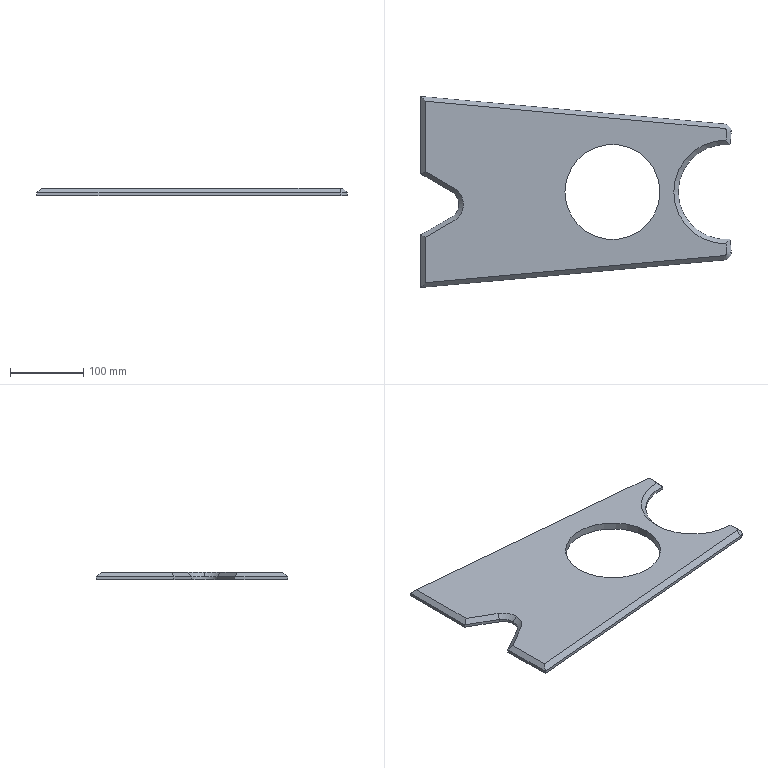Part | SolidWorks | features Chamfer 1, Extrusion 1 | 1 solid | 30 faces | box 424.836 x 261.6 x 10 mm | volume 684949 mm3 | plane 18 | cylinder 7 | cone 5 | commonest cylinder face diameters 130 x4 20 x2 40 x1
STEP:
#1=CARTESIAN_POINT('',(-210.073,-17.,4.));
#2=VERTEX_POINT('',#1);
#3=CARTESIAN_POINT('',(-220.073,0.3205,4.));
#4=VERTEX_POINT('',#3);
#5=CARTESIAN_POINT('',(-230.073,-17.,4.));
#6=DIRECTION('',(0.,0.,1.));
#7=DIRECTION('',(1.,0.,0.));
#8=AXIS2_PLACEMENT_3D('',#5,#6,#7);
#9=CIRCLE('',#8,20.);
#10=EDGE_CURVE('',#2,#4,#9,.T.);
#11=ORIENTED_EDGE('',*,*,#10,.F.);
#12=CARTESIAN_POINT('',(-204.073,-17.,10.));
#13=VERTEX_POINT('',#12);
#14=CARTESIAN_POINT('',(-204.073,-17.,10.));
#15=DIRECTION('',(0.7071,0.,0.7071));
#16=VECTOR('',#15,1000.);
#17=LINE('',#14,#16);
#18=EDGE_CURVE('',#2,#13,#17,.T.);
#19=ORIENTED_EDGE('',*,*,#18,.T.);
#20=CARTESIAN_POINT('',(-217.073,5.517,10.));
#21=VERTEX_POINT('',#20);
#22=CARTESIAN_POINT('',(-230.073,-17.,10.));
#23=DIRECTION('',(0.,0.,-1.));
#24=DIRECTION('',(1.,0.,0.));
#25=AXIS2_PLACEMENT_3D('',#22,#23,#24);
#26=CIRCLE('',#25,26.);
#27=EDGE_CURVE('',#21,#13,#26,.T.);
#28=ORIENTED_EDGE('',*,*,#27,.F.);
#29=CARTESIAN_POINT('',(-217.073,5.517,10.));
#30=DIRECTION('',(-0.3536,-0.6124,-0.7071));
#31=VECTOR('',#30,1000.);
#32=LINE('',#29,#31);
#33=EDGE_CURVE('',#21,#4,#32,.T.);
#34=ORIENTED_EDGE('',*,*,#33,.T.);
#35=EDGE_LOOP('',(#11,#19,#28,#34));
#36=FACE_OUTER_BOUND('',#35,.T.);
#37=CARTESIAN_POINT('',(-230.073,-17.,10.));
#38=DIRECTION('',(0.,0.,1.));
#39=DIRECTION('',(1.,0.,0.));
#40=AXIS2_PLACEMENT_3D('',#37,#38,#39);
#41=CONICAL_SURFACE('',#40,26.,0.7854);
#42=ADVANCED_FACE('',(#36),#41,.F.);
#43=CARTESIAN_POINT('',(-65.,0.,10.));
#44=VERTEX_POINT('',#43);
#45=CARTESIAN_POINT('',(65.,0.,10.));
#46=VERTEX_POINT('',#45);
#47=CARTESIAN_POINT('',(0.,0.,10.));
#48=DIRECTION('',(0.,0.,1.));
#49=DIRECTION('',(1.,0.,0.));
#50=AXIS2_PLACEMENT_3D('',#47,#48,#49);
#51=CIRCLE('',#50,65.);
#52=EDGE_CURVE('',#44,#46,#51,.T.);
#53=ORIENTED_EDGE('',*,*,#52,.T.);
#54=CARTESIAN_POINT('',(65.,0.,0.));
#55=VERTEX_POINT('',#54);
#56=CARTESIAN_POINT('',(65.,0.,10.));
#57=DIRECTION('',(0.,0.,-1.));
#58=VECTOR('',#57,1000.);
#59=LINE('',#56,#58);
#60=EDGE_CURVE('',#46,#55,#59,.T.);
#61=ORIENTED_EDGE('',*,*,#60,.T.);
#62=CARTESIAN_POINT('',(-65.,0.,0.));
#63=VERTEX_POINT('',#62);
#64=CARTESIAN_POINT('',(0.,0.,0.));
#65=DIRECTION('',(0.,0.,1.));
#66=DIRECTION('',(1.,0.,0.));
#67=AXIS2_PLACEMENT_3D('',#64,#65,#66);
#68=CIRCLE('',#67,65.);
#69=EDGE_CURVE('',#63,#55,#68,.T.);
#70=ORIENTED_EDGE('',*,*,#69,.F.);
#71=CARTESIAN_POINT('',(-65.,0.,10.));
#72=DIRECTION('',(0.,0.,-1.));
#73=VECTOR('',#72,1000.);
#74=LINE('',#71,#73);
#75=EDGE_CURVE('',#44,#63,#74,.T.);
#76=ORIENTED_EDGE('',*,*,#75,.F.);
#77=EDGE_LOOP('',(#53,#61,#70,#76));
#78=FACE_OUTER_BOUND('',#77,.T.);
#79=CARTESIAN_POINT('',(0.,0.,10.));
#80=DIRECTION('',(0.,0.,-1.));
#81=DIRECTION('',(-1.,0.,0.));
#82=AXIS2_PLACEMENT_3D('',#79,#80,#81);
#83=CYLINDRICAL_SURFACE('',#82,65.);
#84=ADVANCED_FACE('',(#78),#83,.F.);
#85=CARTESIAN_POINT('',(160.911,64.731,4.));
#86=VERTEX_POINT('',#85);
#87=CARTESIAN_POINT('',(90.,0.,4.));
#88=VERTEX_POINT('',#87);
#89=CARTESIAN_POINT('',(155.,0.,4.));
#90=DIRECTION('',(0.,0.,1.));
#91=DIRECTION('',(1.,0.,0.));
#92=AXIS2_PLACEMENT_3D('',#89,#90,#91);
#93=CIRCLE('',#92,65.);
#94=EDGE_CURVE('',#86,#88,#93,.T.);
#95=ORIENTED_EDGE('',*,*,#94,.T.);
#96=CARTESIAN_POINT('',(90.,0.,0.));
#97=VERTEX_POINT('',#96);
#98=CARTESIAN_POINT('',(90.,0.,10.));
#99=DIRECTION('',(0.,0.,-1.));
#100=VECTOR('',#99,1000.);
#101=LINE('',#98,#100);
#102=EDGE_CURVE('',#88,#97,#101,.T.);
#103=ORIENTED_EDGE('',*,*,#102,.T.);
#104=CARTESIAN_POINT('',(160.911,64.731,0.));
#105=VERTEX_POINT('',#104);
#106=CARTESIAN_POINT('',(155.,0.,0.));
#107=DIRECTION('',(0.,0.,-1.));
#108=DIRECTION('',(1.,0.,0.));
#109=AXIS2_PLACEMENT_3D('',#106,#107,#108);
#110=CIRCLE('',#109,65.);
#111=EDGE_CURVE('',#97,#105,#110,.T.);
#112=ORIENTED_EDGE('',*,*,#111,.T.);
#113=CARTESIAN_POINT('',(160.911,64.731,10.));
#114=DIRECTION('',(0.,0.,-1.));
#115=VECTOR('',#114,1000.);
#116=LINE('',#113,#115);
#117=EDGE_CURVE('',#86,#105,#116,.T.);
#118=ORIENTED_EDGE('',*,*,#117,.F.);
#119=EDGE_LOOP('',(#95,#103,#112,#118));
#120=FACE_OUTER_BOUND('',#119,.T.);
#121=CARTESIAN_POINT('',(155.,0.,10.));
#122=DIRECTION('',(0.,0.,-1.));
#123=DIRECTION('',(-1.,0.,0.));
#124=AXIS2_PLACEMENT_3D('',#121,#122,#123);
#125=CYLINDRICAL_SURFACE('',#124,65.);
#126=ADVANCED_FACE('',(#120),#125,.F.);
#127=CARTESIAN_POINT('',(152.898,-87.047,10.));
#128=VERTEX_POINT('',#127);
#129=CARTESIAN_POINT('',(156.52,-82.702,10.));
#130=VERTEX_POINT('',#129);
#131=CARTESIAN_POINT('',(152.536,-83.064,10.));
#132=DIRECTION('',(0.,0.,1.));
#133=DIRECTION('',(1.,0.,0.));
#134=AXIS2_PLACEMENT_3D('',#131,#132,#133);
#135=CIRCLE('',#134,4.);
#136=EDGE_CURVE('',#128,#130,#135,.T.);
#137=ORIENTED_EDGE('',*,*,#136,.T.);
#138=CARTESIAN_POINT('',(155.456,-70.999,10.));
#139=VERTEX_POINT('',#138);
#140=CARTESIAN_POINT('',(154.936,-65.274,10.));
#141=DIRECTION('',(-0.09049,0.9959,0.));
#142=VECTOR('',#141,1000.);
#143=LINE('',#140,#142);
#144=EDGE_CURVE('',#130,#139,#143,.T.);
#145=ORIENTED_EDGE('',*,*,#144,.T.);
#146=CARTESIAN_POINT('',(155.456,70.999,10.));
#147=VERTEX_POINT('',#146);
#148=CARTESIAN_POINT('',(155.,0.,10.));
#149=DIRECTION('',(0.,0.,-1.));
#150=DIRECTION('',(1.,0.,0.));
#151=AXIS2_PLACEMENT_3D('',#148,#149,#150);
#152=CIRCLE('',#151,71.);
#153=EDGE_CURVE('',#139,#147,#152,.T.);
#154=ORIENTED_EDGE('',*,*,#153,.T.);
#155=CARTESIAN_POINT('',(156.52,82.702,10.));
#156=VERTEX_POINT('',#155);
#157=CARTESIAN_POINT('',(156.52,82.702,10.));
#158=DIRECTION('',(0.09049,0.9959,0.));
#159=VECTOR('',#158,1000.);
#160=LINE('',#157,#159);
#161=EDGE_CURVE('',#147,#156,#160,.T.);
#162=ORIENTED_EDGE('',*,*,#161,.T.);
#163=CARTESIAN_POINT('',(152.898,87.047,10.));
#164=VERTEX_POINT('',#163);
#165=CARTESIAN_POINT('',(152.536,83.064,10.));
#166=DIRECTION('',(0.,0.,1.));
#167=DIRECTION('',(1.,0.,0.));
#168=AXIS2_PLACEMENT_3D('',#165,#166,#167);
#169=CIRCLE('',#168,4.);
#170=EDGE_CURVE('',#156,#164,#169,.T.);
#171=ORIENTED_EDGE('',*,*,#170,.T.);
#172=CARTESIAN_POINT('',(-256.3,124.23,10.));
#173=VERTEX_POINT('',#172);
#174=CARTESIAN_POINT('',(-262.843,124.825,10.));
#175=DIRECTION('',(-0.9959,0.09049,0.));
#176=VECTOR('',#175,1000.);
#177=LINE('',#174,#176);
#178=EDGE_CURVE('',#164,#173,#177,.T.);
#179=ORIENTED_EDGE('',*,*,#178,.T.);
#180=CARTESIAN_POINT('',(-256.3,28.164,10.));
#181=VERTEX_POINT('',#180);
#182=CARTESIAN_POINT('',(-256.3,24.7,10.));
#183=DIRECTION('',(0.,-1.,0.));
#184=VECTOR('',#183,1000.);
#185=LINE('',#182,#184);
#186=EDGE_CURVE('',#173,#181,#185,.T.);
#187=ORIENTED_EDGE('',*,*,#186,.T.);
#188=CARTESIAN_POINT('',(-217.073,5.517,10.));
#189=DIRECTION('',(0.866,-0.5,0.));
#190=VECTOR('',#189,1000.);
#191=LINE('',#188,#190);
#192=EDGE_CURVE('',#181,#21,#191,.T.);
#193=ORIENTED_EDGE('',*,*,#192,.T.);
#194=ORIENTED_EDGE('',*,*,#27,.T.);
#195=CARTESIAN_POINT('',(-217.073,-39.517,10.));
#196=VERTEX_POINT('',#195);
#197=CARTESIAN_POINT('',(-230.073,-17.,10.));
#198=DIRECTION('',(0.,0.,-1.));
#199=DIRECTION('',(1.,0.,0.));
#200=AXIS2_PLACEMENT_3D('',#197,#198,#199);
#201=CIRCLE('',#200,26.);
#202=EDGE_CURVE('',#13,#196,#201,.T.);
#203=ORIENTED_EDGE('',*,*,#202,.T.);
#204=CARTESIAN_POINT('',(-256.3,-62.164,10.));
#205=VERTEX_POINT('',#204);
#206=CARTESIAN_POINT('',(-259.3,-63.896,10.));
#207=DIRECTION('',(-0.866,-0.5,0.));
#208=VECTOR('',#207,1000.);
#209=LINE('',#206,#208);
#210=EDGE_CURVE('',#196,#205,#209,.T.);
#211=ORIENTED_EDGE('',*,*,#210,.T.);
#212=CARTESIAN_POINT('',(-256.3,-124.23,10.));
#213=VERTEX_POINT('',#212);
#214=CARTESIAN_POINT('',(-256.3,-130.8,10.));
#215=DIRECTION('',(0.,-1.,0.));
#216=VECTOR('',#215,1000.);
#217=LINE('',#214,#216);
#218=EDGE_CURVE('',#205,#213,#217,.T.);
#219=ORIENTED_EDGE('',*,*,#218,.T.);
#220=CARTESIAN_POINT('',(152.898,-87.047,10.));
#221=DIRECTION('',(0.9959,0.09049,0.));
#222=VECTOR('',#221,1000.);
#223=LINE('',#220,#222);
#224=EDGE_CURVE('',#213,#128,#223,.T.);
#225=ORIENTED_EDGE('',*,*,#224,.T.);
#226=EDGE_LOOP('',(#137,#145,#154,#162,#171,#179,#187,#193,#194,#203,#211,#219,#225));
#227=FACE_OUTER_BOUND('',#226,.T.);
#228=ORIENTED_EDGE('',*,*,#52,.F.);
#229=CARTESIAN_POINT('',(0.,0.,10.));
#230=DIRECTION('',(0.,0.,1.));
#231=DIRECTION('',(1.,0.,0.));
#232=AXIS2_PLACEMENT_3D('',#229,#230,#231);
#233=CIRCLE('',#232,65.);
#234=EDGE_CURVE('',#46,#44,#233,.T.);
#235=ORIENTED_EDGE('',*,*,#234,.F.);
#236=EDGE_LOOP('',(#228,#235));
#237=FACE_BOUND('',#236,.T.);
#238=CARTESIAN_POINT('',(152.536,-83.064,10.));
#239=DIRECTION('',(0.,0.,1.));
#240=DIRECTION('',(1.,0.,0.));
#241=AXIS2_PLACEMENT_3D('',#238,#239,#240);
#242=PLANE('',#241);
#243=ADVANCED_FACE('',(#227,#237),#242,.T.);
#244=CARTESIAN_POINT('',(-262.3,-58.7,0.));
#245=VERTEX_POINT('',#244);
#246=CARTESIAN_POINT('',(-262.3,-130.8,0.));
#247=VERTEX_POINT('',#246);
#248=CARTESIAN_POINT('',(-262.3,-58.7,0.));
#249=DIRECTION('',(0.,-1.,0.));
#250=VECTOR('',#249,1000.);
#251=LINE('',#248,#250);
#252=EDGE_CURVE('',#245,#247,#251,.T.);
#253=ORIENTED_EDGE('',*,*,#252,.F.);
#254=CARTESIAN_POINT('',(-220.073,-34.321,0.));
#255=VERTEX_POINT('',#254);
#256=CARTESIAN_POINT('',(-262.3,-58.7,0.));
#257=DIRECTION('',(-0.866,-0.5,0.));
#258=VECTOR('',#257,1000.);
#259=LINE('',#256,#258);
#260=EDGE_CURVE('',#255,#245,#259,.T.);
#261=ORIENTED_EDGE('',*,*,#260,.F.);
#262=CARTESIAN_POINT('',(-220.073,0.3205,0.));
#263=VERTEX_POINT('',#262);
#264=CARTESIAN_POINT('',(-230.073,-17.,0.));
#265=DIRECTION('',(0.,0.,-1.));
#266=DIRECTION('',(-1.,0.,0.));
#267=AXIS2_PLACEMENT_3D('',#264,#265,#266);
#268=CIRCLE('',#267,20.);
#269=EDGE_CURVE('',#263,#255,#268,.T.);
#270=ORIENTED_EDGE('',*,*,#269,.F.);
#271=CARTESIAN_POINT('',(-262.3,24.7,0.));
#272=VERTEX_POINT('',#271);
#273=CARTESIAN_POINT('',(-262.3,24.7,0.));
#274=DIRECTION('',(0.866,-0.5,0.));
#275=VECTOR('',#274,1000.);
#276=LINE('',#273,#275);
#277=EDGE_CURVE('',#272,#263,#276,.T.);
#278=ORIENTED_EDGE('',*,*,#277,.F.);
#279=CARTESIAN_POINT('',(-262.3,130.8,0.));
#280=VERTEX_POINT('',#279);
#281=CARTESIAN_POINT('',(-262.3,130.8,0.));
#282=DIRECTION('',(0.,-1.,0.));
#283=VECTOR('',#282,1000.);
#284=LINE('',#281,#283);
#285=EDGE_CURVE('',#280,#272,#284,.T.);
#286=ORIENTED_EDGE('',*,*,#285,.F.);
#287=CARTESIAN_POINT('',(153.441,93.023,0.));
#288=VERTEX_POINT('',#287);
#289=CARTESIAN_POINT('',(-262.3,130.8,0.));
#290=DIRECTION('',(-0.9959,0.09049,0.));
#291=VECTOR('',#290,1000.);
#292=LINE('',#289,#291);
#293=EDGE_CURVE('',#288,#280,#292,.T.);
#294=ORIENTED_EDGE('',*,*,#293,.F.);
#295=CARTESIAN_POINT('',(162.495,82.159,0.));
#296=VERTEX_POINT('',#295);
#297=CARTESIAN_POINT('',(152.536,83.064,0.));
#298=DIRECTION('',(0.,0.,1.));
#299=DIRECTION('',(-1.,0.,0.));
#300=AXIS2_PLACEMENT_3D('',#297,#298,#299);
#301=CIRCLE('',#300,10.);
#302=EDGE_CURVE('',#296,#288,#301,.T.);
#303=ORIENTED_EDGE('',*,*,#302,.F.);
#304=CARTESIAN_POINT('',(162.495,82.159,0.));
#305=DIRECTION('',(0.09049,0.9959,0.));
#306=VECTOR('',#305,1000.);
#307=LINE('',#304,#306);
#308=EDGE_CURVE('',#105,#296,#307,.T.);
#309=ORIENTED_EDGE('',*,*,#308,.F.);
#310=ORIENTED_EDGE('',*,*,#111,.F.);
#311=CARTESIAN_POINT('',(160.911,-64.731,0.));
#312=VERTEX_POINT('',#311);
#313=CARTESIAN_POINT('',(155.,0.,0.));
#314=DIRECTION('',(0.,0.,-1.));
#315=DIRECTION('',(1.,0.,0.));
#316=AXIS2_PLACEMENT_3D('',#313,#314,#315);
#317=CIRCLE('',#316,65.);
#318=EDGE_CURVE('',#312,#97,#317,.T.);
#319=ORIENTED_EDGE('',*,*,#318,.F.);
#320=CARTESIAN_POINT('',(162.495,-82.159,0.));
#321=VERTEX_POINT('',#320);
#322=CARTESIAN_POINT('',(162.495,-82.159,0.));
#323=DIRECTION('',(-0.09049,0.9959,0.));
#324=VECTOR('',#323,1000.);
#325=LINE('',#322,#324);
#326=EDGE_CURVE('',#321,#312,#325,.T.);
#327=ORIENTED_EDGE('',*,*,#326,.F.);
#328=CARTESIAN_POINT('',(153.441,-93.023,0.));
#329=VERTEX_POINT('',#328);
#330=CARTESIAN_POINT('',(152.536,-83.064,0.));
#331=DIRECTION('',(0.,0.,1.));
#332=DIRECTION('',(1.,0.,0.));
#333=AXIS2_PLACEMENT_3D('',#330,#331,#332);
#334=CIRCLE('',#333,10.);
#335=EDGE_CURVE('',#329,#321,#334,.T.);
#336=ORIENTED_EDGE('',*,*,#335,.F.);
#337=CARTESIAN_POINT('',(-262.3,-130.8,0.));
#338=DIRECTION('',(0.9959,0.09049,0.));
#339=VECTOR('',#338,1000.);
#340=LINE('',#337,#339);
#341=EDGE_CURVE('',#247,#329,#340,.T.);
#342=ORIENTED_EDGE('',*,*,#341,.F.);
#343=EDGE_LOOP('',(#253,#261,#270,#278,#286,#294,#303,#309,#310,#319,#327,#336,#342));
#344=FACE_OUTER_BOUND('',#343,.T.);
#345=ORIENTED_EDGE('',*,*,#69,.T.);
#346=CARTESIAN_POINT('',(0.,0.,0.));
#347=DIRECTION('',(0.,0.,1.));
#348=DIRECTION('',(1.,0.,0.));
#349=AXIS2_PLACEMENT_3D('',#346,#347,#348);
#350=CIRCLE('',#349,65.);
#351=EDGE_CURVE('',#55,#63,#350,.T.);
#352=ORIENTED_EDGE('',*,*,#351,.T.);
#353=EDGE_LOOP('',(#345,#352));
#354=FACE_BOUND('',#353,.T.);
#355=CARTESIAN_POINT('',(152.536,-83.064,0.));
#356=DIRECTION('',(0.,0.,1.));
#357=DIRECTION('',(1.,0.,0.));
#358=AXIS2_PLACEMENT_3D('',#355,#356,#357);
#359=PLANE('',#358);
#360=ADVANCED_FACE('',(#344,#354),#359,.F.);
#361=CARTESIAN_POINT('',(-262.3,-130.8,4.));
#362=VERTEX_POINT('',#361);
#363=CARTESIAN_POINT('',(-262.3,-130.8,10.));
#364=DIRECTION('',(0.,0.,-1.));
#365=VECTOR('',#364,1000.);
#366=LINE('',#363,#365);
#367=EDGE_CURVE('',#362,#247,#366,.T.);
#368=ORIENTED_EDGE('',*,*,#367,.F.);
#369=CARTESIAN_POINT('',(-262.3,-58.7,4.));
#370=VERTEX_POINT('',#369);
#371=CARTESIAN_POINT('',(-262.3,-58.7,4.));
#372=DIRECTION('',(0.,1.,0.));
#373=VECTOR('',#372,1000.);
#374=LINE('',#371,#373);
#375=EDGE_CURVE('',#362,#370,#374,.T.);
#376=ORIENTED_EDGE('',*,*,#375,.T.);
#377=CARTESIAN_POINT('',(-262.3,-58.7,10.));
#378=DIRECTION('',(0.,0.,-1.));
#379=VECTOR('',#378,1000.);
#380=LINE('',#377,#379);
#381=EDGE_CURVE('',#370,#245,#380,.T.);
#382=ORIENTED_EDGE('',*,*,#381,.T.);
#383=ORIENTED_EDGE('',*,*,#252,.T.);
#384=EDGE_LOOP('',(#368,#376,#382,#383));
#385=FACE_OUTER_BOUND('',#384,.T.);
#386=CARTESIAN_POINT('',(-262.3,-58.7,10.));
#387=DIRECTION('',(1.,0.,0.));
#388=DIRECTION('',(0.,1.,0.));
#389=AXIS2_PLACEMENT_3D('',#386,#387,#388);
#390=PLANE('',#389);
#391=ADVANCED_FACE('',(#385),#390,.F.);
#392=CARTESIAN_POINT('',(153.441,-93.023,4.));
#393=VERTEX_POINT('',#392);
#394=CARTESIAN_POINT('',(153.441,-93.023,10.));
#395=DIRECTION('',(0.,0.,-1.));
#396=VECTOR('',#395,1000.);
#397=LINE('',#394,#396);
#398=EDGE_CURVE('',#393,#329,#397,.T.);
#399=ORIENTED_EDGE('',*,*,#398,.F.);
#400=CARTESIAN_POINT('',(-262.3,-130.8,4.));
#401=DIRECTION('',(-0.9959,-0.09049,0.));
#402=VECTOR('',#401,1000.);
#403=LINE('',#400,#402);
#404=EDGE_CURVE('',#393,#362,#403,.T.);
#405=ORIENTED_EDGE('',*,*,#404,.T.);
#406=ORIENTED_EDGE('',*,*,#367,.T.);
#407=ORIENTED_EDGE('',*,*,#341,.T.);
#408=EDGE_LOOP('',(#399,#405,#406,#407));
#409=FACE_OUTER_BOUND('',#408,.T.);
#410=CARTESIAN_POINT('',(-262.3,-130.8,10.));
#411=DIRECTION('',(-0.09049,0.9959,0.));
#412=DIRECTION('',(-0.9959,-0.09049,0.));
#413=AXIS2_PLACEMENT_3D('',#410,#411,#412);
#414=PLANE('',#413);
#415=ADVANCED_FACE('',(#409),#414,.F.);
#416=CARTESIAN_POINT('',(162.495,-82.159,4.));
#417=VERTEX_POINT('',#416);
#418=CARTESIAN_POINT('',(162.495,-82.159,10.));
#419=DIRECTION('',(0.,0.,-1.));
#420=VECTOR('',#419,1000.);
#421=LINE('',#418,#420);
#422=EDGE_CURVE('',#417,#321,#421,.T.);
#423=ORIENTED_EDGE('',*,*,#422,.F.);
#424=CARTESIAN_POINT('',(152.536,-83.064,4.));
#425=DIRECTION('',(0.,0.,-1.));
#426=DIRECTION('',(1.,0.,0.));
#427=AXIS2_PLACEMENT_3D('',#424,#425,#426);
#428=CIRCLE('',#427,10.);
#429=EDGE_CURVE('',#417,#393,#428,.T.);
#430=ORIENTED_EDGE('',*,*,#429,.T.);
#431=ORIENTED_EDGE('',*,*,#398,.T.);
#432=ORIENTED_EDGE('',*,*,#335,.T.);
#433=EDGE_LOOP('',(#423,#430,#431,#432));
#434=FACE_OUTER_BOUND('',#433,.T.);
#435=CARTESIAN_POINT('',(152.536,-83.064,10.));
#436=DIRECTION('',(0.,0.,-1.));
#437=DIRECTION('',(-1.,0.,0.));
#438=AXIS2_PLACEMENT_3D('',#435,#436,#437);
#439=CYLINDRICAL_SURFACE('',#438,10.);
#440=ADVANCED_FACE('',(#434),#439,.T.);
#441=CARTESIAN_POINT('',(160.911,-64.731,4.));
#442=VERTEX_POINT('',#441);
#443=CARTESIAN_POINT('',(160.911,-64.731,10.));
#444=DIRECTION('',(0.,0.,-1.));
#445=VECTOR('',#444,1000.);
#446=LINE('',#443,#445);
#447=EDGE_CURVE('',#442,#312,#446,.T.);
#448=ORIENTED_EDGE('',*,*,#447,.F.);
#449=CARTESIAN_POINT('',(162.495,-82.159,4.));
#450=DIRECTION('',(0.09049,-0.9959,0.));
#451=VECTOR('',#450,1000.);
#452=LINE('',#449,#451);
#453=EDGE_CURVE('',#442,#417,#452,.T.);
#454=ORIENTED_EDGE('',*,*,#453,.T.);
#455=ORIENTED_EDGE('',*,*,#422,.T.);
#456=ORIENTED_EDGE('',*,*,#326,.T.);
#457=EDGE_LOOP('',(#448,#454,#455,#456));
#458=FACE_OUTER_BOUND('',#457,.T.);
#459=CARTESIAN_POINT('',(162.495,-82.159,10.));
#460=DIRECTION('',(-0.9959,-0.09049,0.));
#461=DIRECTION('',(0.09049,-0.9959,0.));
#462=AXIS2_PLACEMENT_3D('',#459,#460,#461);
#463=PLANE('',#462);
#464=ADVANCED_FACE('',(#458),#463,.F.);
#465=ORIENTED_EDGE('',*,*,#102,.F.);
#466=CARTESIAN_POINT('',(155.,0.,4.));
#467=DIRECTION('',(0.,0.,1.));
#468=DIRECTION('',(1.,0.,0.));
#469=AXIS2_PLACEMENT_3D('',#466,#467,#468);
#470=CIRCLE('',#469,65.);
#471=EDGE_CURVE('',#88,#442,#470,.T.);
#472=ORIENTED_EDGE('',*,*,#471,.T.);
#473=ORIENTED_EDGE('',*,*,#447,.T.);
#474=ORIENTED_EDGE('',*,*,#318,.T.);
#475=EDGE_LOOP('',(#465,#472,#473,#474));
#476=FACE_OUTER_BOUND('',#475,.T.);
#477=CARTESIAN_POINT('',(155.,0.,10.));
#478=DIRECTION('',(0.,0.,-1.));
#479=DIRECTION('',(-1.,0.,0.));
#480=AXIS2_PLACEMENT_3D('',#477,#478,#479);
#481=CYLINDRICAL_SURFACE('',#480,65.);
#482=ADVANCED_FACE('',(#476),#481,.F.);
#483=CARTESIAN_POINT('',(162.495,82.159,4.));
#484=VERTEX_POINT('',#483);
#485=CARTESIAN_POINT('',(162.495,82.159,10.));
#486=DIRECTION('',(0.,0.,-1.));
#487=VECTOR('',#486,1000.);
#488=LINE('',#485,#487);
#489=EDGE_CURVE('',#484,#296,#488,.T.);
#490=ORIENTED_EDGE('',*,*,#489,.F.);
#491=CARTESIAN_POINT('',(160.911,64.731,4.));
#492=DIRECTION('',(-0.09049,-0.9959,0.));
#493=VECTOR('',#492,1000.);
#494=LINE('',#491,#493);
#495=EDGE_CURVE('',#484,#86,#494,.T.);
#496=ORIENTED_EDGE('',*,*,#495,.T.);
#497=ORIENTED_EDGE('',*,*,#117,.T.);
#498=ORIENTED_EDGE('',*,*,#308,.T.);
#499=EDGE_LOOP('',(#490,#496,#497,#498));
#500=FACE_OUTER_BOUND('',#499,.T.);
#501=CARTESIAN_POINT('',(162.495,82.159,10.));
#502=DIRECTION('',(-0.9959,0.09049,0.));
#503=DIRECTION('',(-0.09049,-0.9959,0.));
#504=AXIS2_PLACEMENT_3D('',#501,#502,#503);
#505=PLANE('',#504);
#506=ADVANCED_FACE('',(#500),#505,.F.);
#507=CARTESIAN_POINT('',(153.441,93.023,4.));
#508=VERTEX_POINT('',#507);
#509=CARTESIAN_POINT('',(153.441,93.023,10.));
#510=DIRECTION('',(0.,0.,-1.));
#511=VECTOR('',#510,1000.);
#512=LINE('',#509,#511);
#513=EDGE_CURVE('',#508,#288,#512,.T.);
#514=ORIENTED_EDGE('',*,*,#513,.F.);
#515=CARTESIAN_POINT('',(152.536,83.064,4.));
#516=DIRECTION('',(0.,0.,-1.));
#517=DIRECTION('',(1.,0.,0.));
#518=AXIS2_PLACEMENT_3D('',#515,#516,#517);
#519=CIRCLE('',#518,10.);
#520=EDGE_CURVE('',#508,#484,#519,.T.);
#521=ORIENTED_EDGE('',*,*,#520,.T.);
#522=ORIENTED_EDGE('',*,*,#489,.T.);
#523=ORIENTED_EDGE('',*,*,#302,.T.);
#524=EDGE_LOOP('',(#514,#521,#522,#523));
#525=FACE_OUTER_BOUND('',#524,.T.);
#526=CARTESIAN_POINT('',(152.536,83.064,10.));
#527=DIRECTION('',(0.,0.,-1.));
#528=DIRECTION('',(-1.,0.,0.));
#529=AXIS2_PLACEMENT_3D('',#526,#527,#528);
#530=CYLINDRICAL_SURFACE('',#529,10.);
#531=ADVANCED_FACE('',(#525),#530,.T.);
#532=CARTESIAN_POINT('',(-262.3,130.8,4.));
#533=VERTEX_POINT('',#532);
#534=CARTESIAN_POINT('',(-262.3,130.8,10.));
#535=DIRECTION('',(0.,0.,-1.));
#536=VECTOR('',#535,1000.);
#537=LINE('',#534,#536);
#538=EDGE_CURVE('',#533,#280,#537,.T.);
#539=ORIENTED_EDGE('',*,*,#538,.F.);
#540=CARTESIAN_POINT('',(153.441,93.023,4.));
#541=DIRECTION('',(0.9959,-0.09049,0.));
#542=VECTOR('',#541,1000.);
#543=LINE('',#540,#542);
#544=EDGE_CURVE('',#533,#508,#543,.T.);
#545=ORIENTED_EDGE('',*,*,#544,.T.);
#546=ORIENTED_EDGE('',*,*,#513,.T.);
#547=ORIENTED_EDGE('',*,*,#293,.T.);
#548=EDGE_LOOP('',(#539,#545,#546,#547));
#549=FACE_OUTER_BOUND('',#548,.T.);
#550=CARTESIAN_POINT('',(-262.3,130.8,10.));
#551=DIRECTION('',(-0.09049,-0.9959,0.));
#552=DIRECTION('',(0.9959,-0.09049,0.));
#553=AXIS2_PLACEMENT_3D('',#550,#551,#552);
#554=PLANE('',#553);
#555=ADVANCED_FACE('',(#549),#554,.F.);
#556=CARTESIAN_POINT('',(-262.3,24.7,4.));
#557=VERTEX_POINT('',#556);
#558=CARTESIAN_POINT('',(-262.3,24.7,10.));
#559=DIRECTION('',(0.,0.,-1.));
#560=VECTOR('',#559,1000.);
#561=LINE('',#558,#560);
#562=EDGE_CURVE('',#557,#272,#561,.T.);
#563=ORIENTED_EDGE('',*,*,#562,.F.);
#564=CARTESIAN_POINT('',(-262.3,130.8,4.));
#565=DIRECTION('',(0.,1.,0.));
#566=VECTOR('',#565,1000.);
#567=LINE('',#564,#566);
#568=EDGE_CURVE('',#557,#533,#567,.T.);
#569=ORIENTED_EDGE('',*,*,#568,.T.);
#570=ORIENTED_EDGE('',*,*,#538,.T.);
#571=ORIENTED_EDGE('',*,*,#285,.T.);
#572=EDGE_LOOP('',(#563,#569,#570,#571));
#573=FACE_OUTER_BOUND('',#572,.T.);
#574=CARTESIAN_POINT('',(-262.3,130.8,10.));
#575=DIRECTION('',(1.,0.,0.));
#576=DIRECTION('',(0.,1.,0.));
#577=AXIS2_PLACEMENT_3D('',#574,#575,#576);
#578=PLANE('',#577);
#579=ADVANCED_FACE('',(#573),#578,.F.);
#580=CARTESIAN_POINT('',(-220.073,0.3205,10.));
#581=DIRECTION('',(0.,0.,-1.));
#582=VECTOR('',#581,1000.);
#583=LINE('',#580,#582);
#584=EDGE_CURVE('',#4,#263,#583,.T.);
#585=ORIENTED_EDGE('',*,*,#584,.F.);
#586=CARTESIAN_POINT('',(-262.3,24.7,4.));
#587=DIRECTION('',(-0.866,0.5,0.));
#588=VECTOR('',#587,1000.);
#589=LINE('',#586,#588);
#590=EDGE_CURVE('',#4,#557,#589,.T.);
#591=ORIENTED_EDGE('',*,*,#590,.T.);
#592=ORIENTED_EDGE('',*,*,#562,.T.);
#593=ORIENTED_EDGE('',*,*,#277,.T.);
#594=EDGE_LOOP('',(#585,#591,#592,#593));
#595=FACE_OUTER_BOUND('',#594,.T.);
#596=CARTESIAN_POINT('',(-262.3,24.7,10.));
#597=DIRECTION('',(0.5,0.866,0.));
#598=DIRECTION('',(-0.866,0.5,0.));
#599=AXIS2_PLACEMENT_3D('',#596,#597,#598);
#600=PLANE('',#599);
#601=ADVANCED_FACE('',(#595),#600,.F.);
#602=CARTESIAN_POINT('',(-220.073,-34.321,4.));
#603=VERTEX_POINT('',#602);
#604=CARTESIAN_POINT('',(-220.073,-34.321,10.));
#605=DIRECTION('',(0.,0.,-1.));
#606=VECTOR('',#605,1000.);
#607=LINE('',#604,#606);
#608=EDGE_CURVE('',#603,#255,#607,.T.);
#609=ORIENTED_EDGE('',*,*,#608,.F.);
#610=CARTESIAN_POINT('',(-230.073,-17.,4.));
#611=DIRECTION('',(0.,0.,1.));
#612=DIRECTION('',(1.,0.,0.));
#613=AXIS2_PLACEMENT_3D('',#610,#611,#612);
#614=CIRCLE('',#613,20.);
#615=EDGE_CURVE('',#603,#2,#614,.T.);
#616=ORIENTED_EDGE('',*,*,#615,.T.);
#617=ORIENTED_EDGE('',*,*,#10,.T.);
#618=ORIENTED_EDGE('',*,*,#584,.T.);
#619=ORIENTED_EDGE('',*,*,#269,.T.);
#620=EDGE_LOOP('',(#609,#616,#617,#618,#619));
#621=FACE_OUTER_BOUND('',#620,.T.);
#622=CARTESIAN_POINT('',(-230.073,-17.,10.));
#623=DIRECTION('',(0.,0.,-1.));
#624=DIRECTION('',(-1.,0.,0.));
#625=AXIS2_PLACEMENT_3D('',#622,#623,#624);
#626=CYLINDRICAL_SURFACE('',#625,20.);
#627=ADVANCED_FACE('',(#621),#626,.F.);
#628=ORIENTED_EDGE('',*,*,#381,.F.);
#629=CARTESIAN_POINT('',(-220.073,-34.321,4.));
#630=DIRECTION('',(0.866,0.5,0.));
#631=VECTOR('',#630,1000.);
#632=LINE('',#629,#631);
#633=EDGE_CURVE('',#370,#603,#632,.T.);
#634=ORIENTED_EDGE('',*,*,#633,.T.);
#635=ORIENTED_EDGE('',*,*,#608,.T.);
#636=ORIENTED_EDGE('',*,*,#260,.T.);
#637=EDGE_LOOP('',(#628,#634,#635,#636));
#638=FACE_OUTER_BOUND('',#637,.T.);
#639=CARTESIAN_POINT('',(-262.3,-58.7,10.));
#640=DIRECTION('',(0.5,-0.866,0.));
#641=DIRECTION('',(0.866,0.5,0.));
#642=AXIS2_PLACEMENT_3D('',#639,#640,#641);
#643=PLANE('',#642);
#644=ADVANCED_FACE('',(#638),#643,.F.);
#645=ORIENTED_EDGE('',*,*,#60,.F.);
#646=ORIENTED_EDGE('',*,*,#234,.T.);
#647=ORIENTED_EDGE('',*,*,#75,.T.);
#648=ORIENTED_EDGE('',*,*,#351,.F.);
#649=EDGE_LOOP('',(#645,#646,#647,#648));
#650=FACE_OUTER_BOUND('',#649,.T.);
#651=CARTESIAN_POINT('',(0.,0.,10.));
#652=DIRECTION('',(0.,0.,-1.));
#653=DIRECTION('',(-1.,0.,0.));
#654=AXIS2_PLACEMENT_3D('',#651,#652,#653);
#655=CYLINDRICAL_SURFACE('',#654,65.);
#656=ADVANCED_FACE('',(#650),#655,.F.);
#657=CARTESIAN_POINT('',(-283.822,12.274,-17.522));
#658=DIRECTION('',(0.6547,0.378,0.6547));
#659=VECTOR('',#658,1000.);
#660=LINE('',#657,#659);
#661=EDGE_CURVE('',#557,#181,#660,.T.);
#662=ORIENTED_EDGE('',*,*,#661,.F.);
#663=ORIENTED_EDGE('',*,*,#590,.F.);
#664=ORIENTED_EDGE('',*,*,#33,.F.);
#665=ORIENTED_EDGE('',*,*,#192,.F.);
#666=EDGE_LOOP('',(#662,#663,#664,#665));
#667=FACE_OUTER_BOUND('',#666,.T.);
#668=CARTESIAN_POINT('',(98.49,-176.674,10.));
#669=DIRECTION('',(-0.3536,-0.6124,0.7071));
#670=DIRECTION('',(0.,-0.7559,-0.6547));
#671=AXIS2_PLACEMENT_3D('',#668,#669,#670);
#672=PLANE('',#671);
#673=ADVANCED_FACE('',(#667),#672,.T.);
#674=ORIENTED_EDGE('',*,*,#18,.F.);
#675=ORIENTED_EDGE('',*,*,#615,.F.);
#676=CARTESIAN_POINT('',(-217.073,-39.517,10.));
#677=DIRECTION('',(-0.3536,0.6124,-0.7071));
#678=VECTOR('',#677,1000.);
#679=LINE('',#676,#678);
#680=EDGE_CURVE('',#196,#603,#679,.T.);
#681=ORIENTED_EDGE('',*,*,#680,.F.);
#682=ORIENTED_EDGE('',*,*,#202,.F.);
#683=EDGE_LOOP('',(#674,#675,#681,#682));
#684=FACE_OUTER_BOUND('',#683,.T.);
#685=CARTESIAN_POINT('',(-230.073,-17.,10.));
#686=DIRECTION('',(0.,0.,1.));
#687=DIRECTION('',(1.,0.,0.));
#688=AXIS2_PLACEMENT_3D('',#685,#686,#687);
#689=CONICAL_SURFACE('',#688,26.,0.7854);
#690=ADVANCED_FACE('',(#684),#689,.F.);
#691=ORIENTED_EDGE('',*,*,#661,.T.);
#692=ORIENTED_EDGE('',*,*,#186,.F.);
#693=CARTESIAN_POINT('',(-110.512,-35.406,155.788));
#694=DIRECTION('',(0.5591,-0.6122,0.5591));
#695=VECTOR('',#694,1000.);
#696=LINE('',#693,#695);
#697=EDGE_CURVE('',#533,#173,#696,.T.);
#698=ORIENTED_EDGE('',*,*,#697,.F.);
#699=ORIENTED_EDGE('',*,*,#568,.F.);
#700=EDGE_LOOP('',(#691,#692,#698,#699));
#701=FACE_OUTER_BOUND('',#700,.T.);
#702=CARTESIAN_POINT('',(-256.3,-83.064,10.));
#703=DIRECTION('',(-0.7071,0.,0.7071));
#704=DIRECTION('',(0.7071,0.,0.7071));
#705=AXIS2_PLACEMENT_3D('',#702,#703,#704);
#706=PLANE('',#705);
#707=ADVANCED_FACE('',(#701),#706,.T.);
#708=ORIENTED_EDGE('',*,*,#680,.T.);
#709=ORIENTED_EDGE('',*,*,#633,.F.);
#710=CARTESIAN_POINT('',(-171.278,-111.252,95.022));
#711=DIRECTION('',(-0.6547,0.378,-0.6547));
#712=VECTOR('',#711,1000.);
#713=LINE('',#710,#712);
#714=EDGE_CURVE('',#205,#370,#713,.T.);
#715=ORIENTED_EDGE('',*,*,#714,.F.);
#716=ORIENTED_EDGE('',*,*,#210,.F.);
#717=EDGE_LOOP('',(#708,#709,#715,#716));
#718=FACE_OUTER_BOUND('',#717,.T.);
#719=CARTESIAN_POINT('',(41.277,109.642,10.));
#720=DIRECTION('',(-0.3536,0.6124,0.7071));
#721=DIRECTION('',(0.,-0.7559,0.6547));
#722=AXIS2_PLACEMENT_3D('',#719,#720,#721);
#723=PLANE('',#722);
#724=ADVANCED_FACE('',(#718),#723,.T.);
#725=ORIENTED_EDGE('',*,*,#697,.T.);
#726=ORIENTED_EDGE('',*,*,#178,.F.);
#727=CARTESIAN_POINT('',(153.441,93.023,4.));
#728=DIRECTION('',(-0.06399,-0.7042,0.7071));
#729=VECTOR('',#728,1000.);
#730=LINE('',#727,#729);
#731=EDGE_CURVE('',#508,#164,#730,.T.);
#732=ORIENTED_EDGE('',*,*,#731,.F.);
#733=ORIENTED_EDGE('',*,*,#544,.F.);
#734=EDGE_LOOP('',(#725,#726,#732,#733));
#735=FACE_OUTER_BOUND('',#734,.T.);
#736=CARTESIAN_POINT('',(167.87,85.687,10.));
#737=DIRECTION('',(0.06399,0.7042,0.7071));
#738=DIRECTION('',(0.,-0.7086,0.7057));
#739=AXIS2_PLACEMENT_3D('',#736,#737,#738);
#740=PLANE('',#739);
#741=ADVANCED_FACE('',(#735),#740,.T.);
#742=ORIENTED_EDGE('',*,*,#714,.T.);
#743=ORIENTED_EDGE('',*,*,#375,.F.);
#744=CARTESIAN_POINT('',(-242.209,-108.801,24.091));
#745=DIRECTION('',(-0.5591,-0.6122,-0.5591));
#746=VECTOR('',#745,1000.);
#747=LINE('',#744,#746);
#748=EDGE_CURVE('',#213,#362,#747,.T.);
#749=ORIENTED_EDGE('',*,*,#748,.F.);
#750=ORIENTED_EDGE('',*,*,#218,.F.);
#751=EDGE_LOOP('',(#742,#743,#749,#750));
#752=FACE_OUTER_BOUND('',#751,.T.);
#753=CARTESIAN_POINT('',(-256.3,-83.064,10.));
#754=DIRECTION('',(-0.7071,0.,0.7071));
#755=DIRECTION('',(0.7071,0.,0.7071));
#756=AXIS2_PLACEMENT_3D('',#753,#754,#755);
#757=PLANE('',#756);
#758=ADVANCED_FACE('',(#752),#757,.T.);
#759=ORIENTED_EDGE('',*,*,#731,.T.);
#760=ORIENTED_EDGE('',*,*,#170,.F.);
#761=CARTESIAN_POINT('',(162.495,82.159,4.));
#762=DIRECTION('',(-0.7042,0.06399,0.7071));
#763=VECTOR('',#762,1000.);
#764=LINE('',#761,#763);
#765=EDGE_CURVE('',#484,#156,#764,.T.);
#766=ORIENTED_EDGE('',*,*,#765,.F.);
#767=ORIENTED_EDGE('',*,*,#520,.F.);
#768=EDGE_LOOP('',(#759,#760,#766,#767));
#769=FACE_OUTER_BOUND('',#768,.T.);
#770=CARTESIAN_POINT('',(152.536,83.064,10.));
#771=DIRECTION('',(0.,0.,-1.));
#772=DIRECTION('',(-1.,0.,0.));
#773=AXIS2_PLACEMENT_3D('',#770,#771,#772);
#774=CONICAL_SURFACE('',#773,4.,0.7854);
#775=ADVANCED_FACE('',(#769),#774,.T.);
#776=ORIENTED_EDGE('',*,*,#748,.T.);
#777=ORIENTED_EDGE('',*,*,#404,.F.);
#778=CARTESIAN_POINT('',(152.898,-87.047,10.));
#779=DIRECTION('',(0.06399,-0.7042,-0.7071));
#780=VECTOR('',#779,1000.);
#781=LINE('',#778,#780);
#782=EDGE_CURVE('',#128,#393,#781,.T.);
#783=ORIENTED_EDGE('',*,*,#782,.F.);
#784=ORIENTED_EDGE('',*,*,#224,.F.);
#785=EDGE_LOOP('',(#776,#777,#783,#784));
#786=FACE_OUTER_BOUND('',#785,.T.);
#787=CARTESIAN_POINT('',(152.898,-87.047,10.));
#788=DIRECTION('',(0.06399,-0.7042,0.7071));
#789=DIRECTION('',(0.,-0.7086,-0.7057));
#790=AXIS2_PLACEMENT_3D('',#787,#788,#789);
#791=PLANE('',#790);
#792=ADVANCED_FACE('',(#786),#791,.T.);
#793=ORIENTED_EDGE('',*,*,#765,.T.);
#794=ORIENTED_EDGE('',*,*,#161,.F.);
#795=CARTESIAN_POINT('',(160.911,64.731,4.));
#796=CARTESIAN_POINT('',(159.126,66.874,5.973));
#797=CARTESIAN_POINT('',(157.305,68.961,7.974));
#798=CARTESIAN_POINT('',(155.456,70.999,10.));
#799=B_SPLINE_CURVE_WITH_KNOTS('',3,(#795,#796,#797,#798),.UNSPECIFIED.,.F.,.F.,(4,4),(0.,0.01025),.UNSPECIFIED.);
#800=EDGE_CURVE('',#86,#147,#799,.T.);
#801=ORIENTED_EDGE('',*,*,#800,.F.);
#802=ORIENTED_EDGE('',*,*,#495,.F.);
#803=EDGE_LOOP('',(#793,#794,#801,#802));
#804=FACE_OUTER_BOUND('',#803,.T.);
#805=CARTESIAN_POINT('',(141.548,-82.065,10.));
#806=DIRECTION('',(0.7042,-0.06399,0.7071));
#807=DIRECTION('',(0.7086,0.,-0.7057));
#808=AXIS2_PLACEMENT_3D('',#805,#806,#807);
#809=PLANE('',#808);
#810=ADVANCED_FACE('',(#804),#809,.T.);
#811=ORIENTED_EDGE('',*,*,#782,.T.);
#812=ORIENTED_EDGE('',*,*,#429,.F.);
#813=CARTESIAN_POINT('',(156.52,-82.702,10.));
#814=DIRECTION('',(0.7042,0.06399,-0.7071));
#815=VECTOR('',#814,1000.);
#816=LINE('',#813,#815);
#817=EDGE_CURVE('',#130,#417,#816,.T.);
#818=ORIENTED_EDGE('',*,*,#817,.F.);
#819=ORIENTED_EDGE('',*,*,#136,.F.);
#820=EDGE_LOOP('',(#811,#812,#818,#819));
#821=FACE_OUTER_BOUND('',#820,.T.);
#822=CARTESIAN_POINT('',(152.536,-83.064,10.));
#823=DIRECTION('',(0.,0.,-1.));
#824=DIRECTION('',(-1.,0.,0.));
#825=AXIS2_PLACEMENT_3D('',#822,#823,#824);
#826=CONICAL_SURFACE('',#825,4.,0.7854);
#827=ADVANCED_FACE('',(#821),#826,.T.);
#828=ORIENTED_EDGE('',*,*,#800,.T.);
#829=ORIENTED_EDGE('',*,*,#153,.F.);
#830=CARTESIAN_POINT('',(160.911,-64.731,4.));
#831=CARTESIAN_POINT('',(159.126,-66.874,5.973));
#832=CARTESIAN_POINT('',(157.305,-68.961,7.974));
#833=CARTESIAN_POINT('',(155.456,-70.999,10.));
#834=B_SPLINE_CURVE_WITH_KNOTS('',3,(#830,#831,#832,#833),.UNSPECIFIED.,.F.,.F.,(4,4),(0.,0.01025),.UNSPECIFIED.);
#835=EDGE_CURVE('',#442,#139,#834,.T.);
#836=ORIENTED_EDGE('',*,*,#835,.F.);
#837=ORIENTED_EDGE('',*,*,#471,.F.);
#838=ORIENTED_EDGE('',*,*,#94,.F.);
#839=EDGE_LOOP('',(#828,#829,#836,#837,#838));
#840=FACE_OUTER_BOUND('',#839,.T.);
#841=CARTESIAN_POINT('',(155.,0.,10.));
#842=DIRECTION('',(0.,0.,1.));
#843=DIRECTION('',(1.,0.,0.));
#844=AXIS2_PLACEMENT_3D('',#841,#842,#843);
#845=CONICAL_SURFACE('',#844,71.,0.7854);
#846=ADVANCED_FACE('',(#840),#845,.F.);
#847=ORIENTED_EDGE('',*,*,#817,.T.);
#848=ORIENTED_EDGE('',*,*,#453,.F.);
#849=ORIENTED_EDGE('',*,*,#835,.T.);
#850=ORIENTED_EDGE('',*,*,#144,.F.);
#851=EDGE_LOOP('',(#847,#848,#849,#850));
#852=FACE_OUTER_BOUND('',#851,.T.);
#853=CARTESIAN_POINT('',(156.52,-82.702,10.));
#854=DIRECTION('',(0.7042,0.06399,0.7071));
#855=DIRECTION('',(0.7086,0.,-0.7057));
#856=AXIS2_PLACEMENT_3D('',#853,#854,#855);
#857=PLANE('',#856);
#858=ADVANCED_FACE('',(#852),#857,.T.);
#859=CLOSED_SHELL('',(#42,#84,#126,#243,#360,#391,#415,#440,#464,#482,#506,#531,#555,#579,#601,#627,#644,#656,#673,#690,#707,#724,#741,#758,#775,#792,#810,#827,#846,#858));
#860=MANIFOLD_SOLID_BREP('',#859);
#861=CARTESIAN_POINT('',(0.,0.,0.));
#862=DIRECTION('',(0.,0.,1.));
#863=DIRECTION('',(1.,0.,0.));
#864=AXIS2_PLACEMENT_3D('',#861,#862,#863);
#865=(LENGTH_UNIT()NAMED_UNIT(*)SI_UNIT(.MILLI.,.METRE.));
#866=UNCERTAINTY_MEASURE_WITH_UNIT(LENGTH_MEASURE(0.00001),#865,'','');
#867=(NAMED_UNIT(*)PLANE_ANGLE_UNIT()SI_UNIT($,.RADIAN.));
#868=(NAMED_UNIT(*)SI_UNIT($,.STERADIAN.)SOLID_ANGLE_UNIT());
#869=(GEOMETRIC_REPRESENTATION_CONTEXT(3)GLOBAL_UNCERTAINTY_ASSIGNED_CONTEXT((#866))GLOBAL_UNIT_ASSIGNED_CONTEXT((#865,#867,#868))REPRESENTATION_CONTEXT('',''));
#870=ADVANCED_BREP_SHAPE_REPRESENTATION('',(#860,#864),#869);